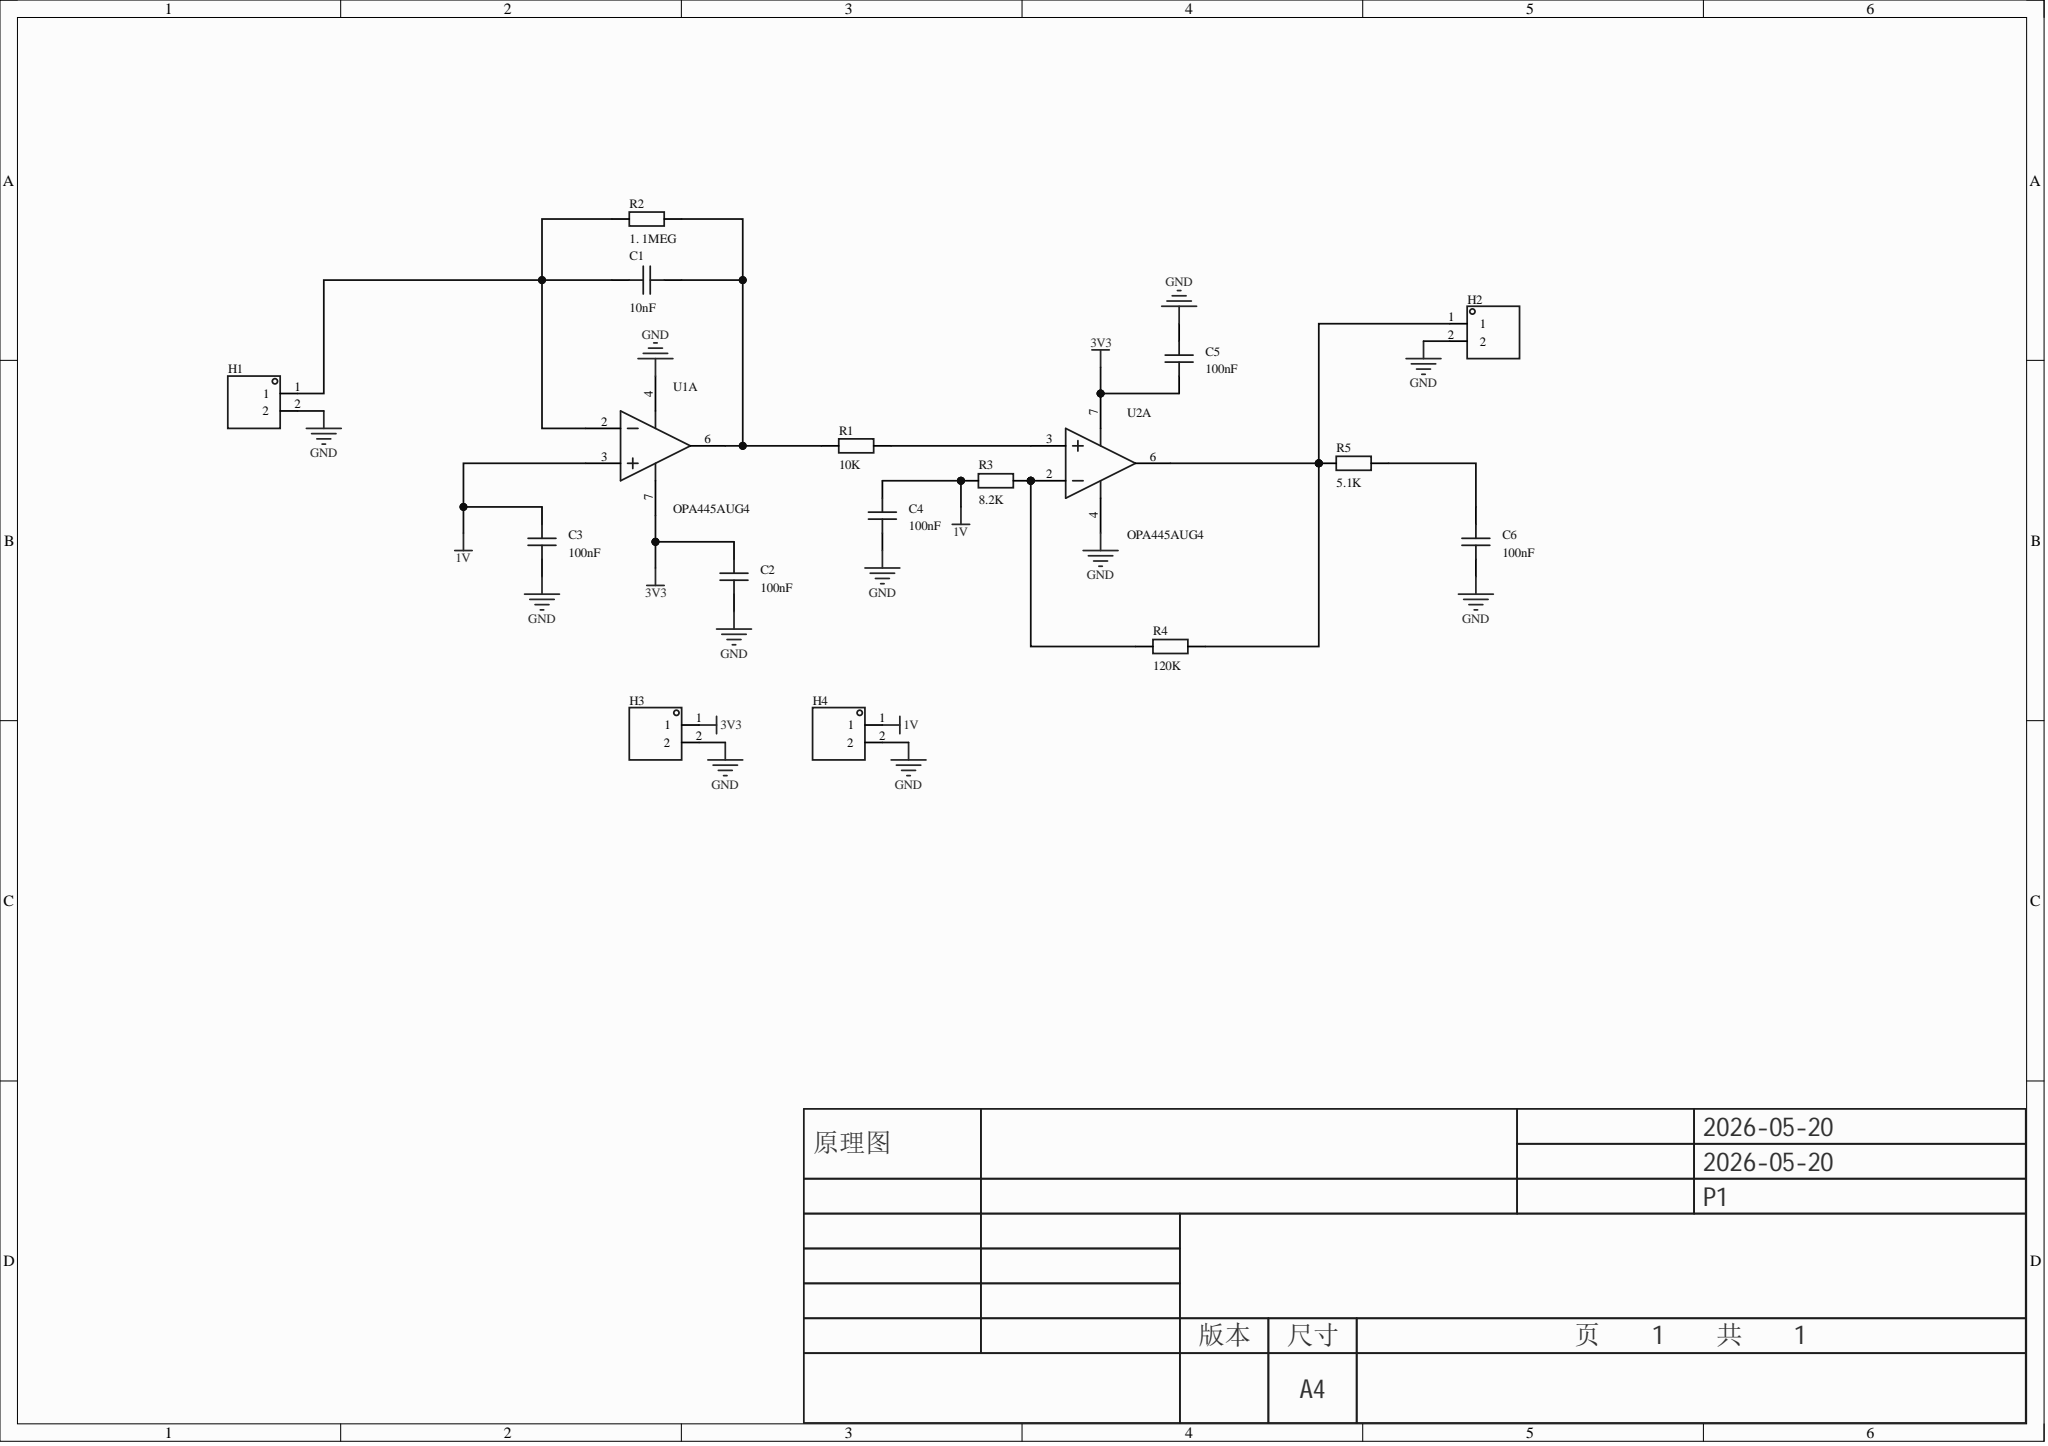Circuit board | Altium Designer | 17 parts | 9 nets
Bill of materials:
Comment,Description,Designator,Footprint,LibRef,Quantity
"10nF","","C1","C0603","CAP_0603","1"
"100nF","","C2, C3, C4, C5, C6","C0603","CAP_0603","5"
"","","H1, H2, H3, H4","HDR-TH_2P-P2.54-V-M-1","HDR-M_2.54_1x2P","4"
"10K","","R1","R0603","Res_0603","1"
"1. 1MEG","","R2","R0603","Res_0603","1"
"8.2K","","R3","R0603","Res_0603","1"
"120K","","R4","R0603","Res_0603","1"
"5.1K","","R5","R0603","Res_0603","1"
"OPA445AUG4","","U1, U2","SOIC-8_L4.9-W3.9-P1.27-LS6.0-BL","OPA445AUG4","2"
Netlist (Protel format):
[
C1
C0603
10nF



]
[
C2
C0603
100nF



]
[
C3
C0603
100nF



]
[
C4
C0603
100nF



]
[
C5
C0603
100nF



]
[
C6
C0603
100nF



]
[
H1
HDR-TH_2P-P2.54-V-M-1




]
[
H2
HDR-TH_2P-P2.54-V-M-1




]
[
H3
HDR-TH_2P-P2.54-V-M-1




]
[
H4
HDR-TH_2P-P2.54-V-M-1




]
[
R1
R0603
10K



]
[
R2
R0603
1. 1MEG



]
[
R3
R0603
8.2K



]
[
R4
R0603
120K



]
[
R5
R0603
5.1K



]
[
U1
SOIC-8_L4.9-W3.9-P1.27-LS6.0-BL
OPA445AUG4



]
[
U2
SOIC-8_L4.9-W3.9-P1.27-LS6.0-BL
OPA445AUG4



]
(
NetR3_2
R3-2
R4-1
U2-2
)
(
NetR1_2
R1-2
U2-3
)
(
NetH2_1
H2-1
R4-2
R5-1
U2-6
)
(
NetC6_1
C6-1
R5-2
)
(
NetC1_2
C1-2
R1-1
R2-2
U1-6
)
(
NetC1_1
C1-1
H1-1
R2-1
U1-2
)
(
GND
C2-1
C3-1
C4-1
C5-1
C6-2
H1-2
H2-2
H3-2
H4-2
U1-4
U2-4
)
(
3V3
C2-2
C5-2
H3-1
U1-7
U2-7
)
(
1V
C3-2
C4-2
H4-1
R3-1
U1-3
)